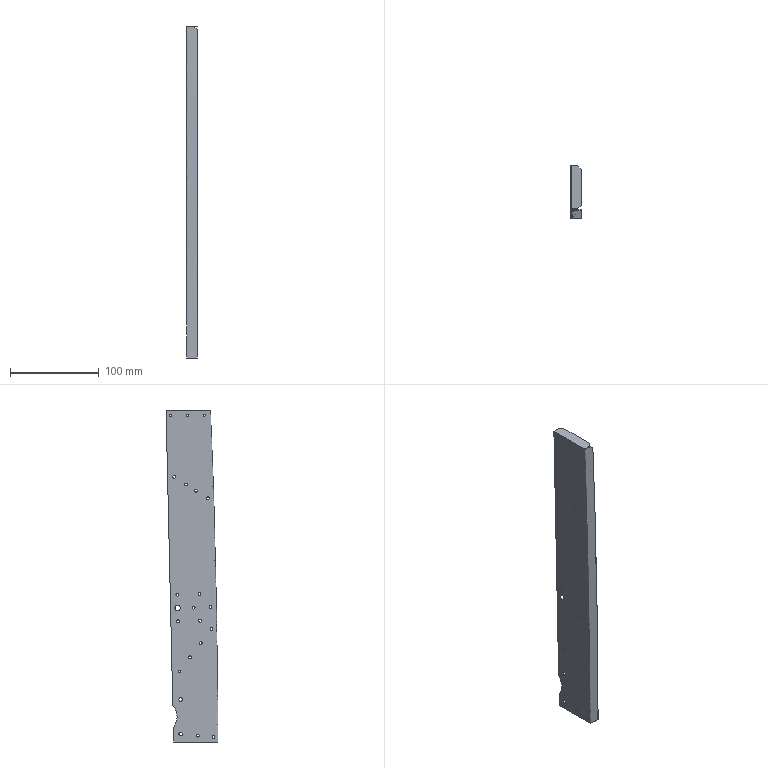Part | SolidWorks | features BaseBody 1 | 1 solid | 59 faces | box 12 x 58.518 x 374.55 mm | volume 10470 mm3 | cylinder 45 | plane 10 | spline 4 | commonest cylinder face diameters 3.2 x32 2.4 x6 4 x4 6.35 x2 36 x1